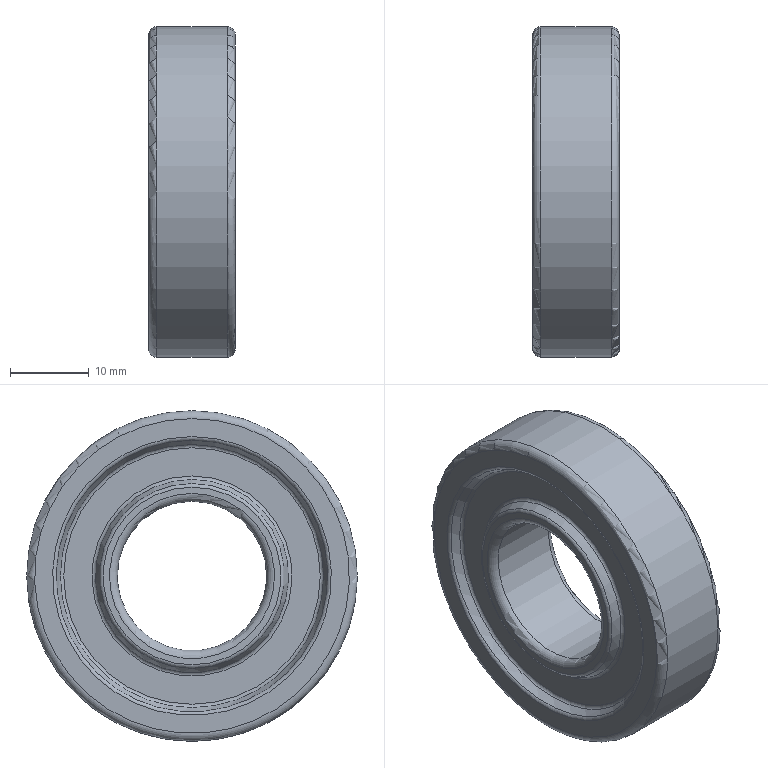Part | STEP file | PL6203ZZA_default | 1 solid | 24 faces | box 11 x 42 x 42 mm | volume 10581 mm3 | torus 12 | plane 6 | cone 4 | cylinder 2 | commonest cylinder face diameters 19 x1 42 x1
STEP:
#1=CARTESIAN_POINT('',(0.,0.,0.));
#2=DIRECTION('',(0.,0.,1.));
#3=DIRECTION('',(1.,0.,0.));
#4=AXIS2_PLACEMENT_3D('',#1,#2,#3);
#5=CARTESIAN_POINT('',(0.,-9.5,20.));
#6=VERTEX_POINT('',#5);
#7=CARTESIAN_POINT('',(0.,-9.5,0.));
#8=DIRECTION('',(-1.,0.,0.));
#9=DIRECTION('',(0.,0.,1.));
#10=AXIS2_PLACEMENT_3D('',#7,#8,#9);
#11=CIRCLE('',#10,20.);
#12=CARTESIAN_POINT('',(1.,-9.5,0.));
#13=DIRECTION('',(-1.,0.,0.));
#14=DIRECTION('',(0.,0.,1.));
#15=AXIS2_PLACEMENT_3D('',#12,#13,#14);
#16=TOROIDAL_SURFACE('',#15,20.,1.);
#17=CARTESIAN_POINT('',(0.,7.854));
#18=DIRECTION('',(1.,0.));
#19=VECTOR('',#18,1.);
#20=LINE('',#17,#19);
#21=(GEOMETRIC_REPRESENTATION_CONTEXT(2)PARAMETRIC_REPRESENTATION_CONTEXT()REPRESENTATION_CONTEXT('',''));
#22=DEFINITIONAL_REPRESENTATION('',(#20),#21);
#23=PCURVE('',#16,#22);
#24=CARTESIAN_POINT('',(0.,8.209,0.));
#25=DIRECTION('',(1.,0.,0.));
#26=DIRECTION('',(0.,0.,-1.));
#27=AXIS2_PLACEMENT_3D('',#24,#25,#26);
#28=PLANE('',#27);
#29=CARTESIAN_POINT('',(-20.,-17.709));
#30=CARTESIAN_POINT('',(-20.,16.932));
#31=CARTESIAN_POINT('',(10.,-0.3885));
#32=CARTESIAN_POINT('',(40.,-17.709));
#33=CARTESIAN_POINT('',(10.,-35.03));
#34=CARTESIAN_POINT('',(-20.,-52.35));
#35=CARTESIAN_POINT('',(-20.,-17.709));
#36=(BOUNDED_CURVE()B_SPLINE_CURVE(2,(#29,#30,#31,#32,#33,#34,#35),.UNSPECIFIED.,.T.,.F.)B_SPLINE_CURVE_WITH_KNOTS((1,2,2,2,2,1),(-2.094,0.,2.094,4.189,6.283,8.378),.UNSPECIFIED.)CURVE()GEOMETRIC_REPRESENTATION_ITEM()RATIONAL_B_SPLINE_CURVE((1.,0.5,1.,0.5,1.,0.5,1.))REPRESENTATION_ITEM(''));
#37=(GEOMETRIC_REPRESENTATION_CONTEXT(2)PARAMETRIC_REPRESENTATION_CONTEXT()REPRESENTATION_CONTEXT('',''));
#38=DEFINITIONAL_REPRESENTATION('',(#36),#37);
#39=PCURVE('',#28,#38);
#40=SURFACE_CURVE('',#11,(#23,#39),.PCURVE_S1.);
#41=EDGE_CURVE('',#6,#6,#40,.T.);
#42=ORIENTED_EDGE('',*,*,#41,.F.);
#43=CARTESIAN_POINT('',(1.,-9.5,21.));
#44=VERTEX_POINT('',#43);
#45=CARTESIAN_POINT('',(1.,-9.5,21.));
#46=CARTESIAN_POINT('',(0.7327,-9.5,21.));
#47=CARTESIAN_POINT('',(0.4723,-9.5,20.915));
#48=CARTESIAN_POINT('',(0.2481,-9.5,20.752));
#49=CARTESIAN_POINT('',(0.085,-9.5,20.528));
#50=CARTESIAN_POINT('',(0.,-9.5,20.267));
#51=CARTESIAN_POINT('',(0.,-9.5,20.));
#52=(BOUNDED_CURVE()B_SPLINE_CURVE(6,(#45,#46,#47,#48,#49,#50,#51),.UNSPECIFIED.,.F.,.F.)B_SPLINE_CURVE_WITH_KNOTS((7,7),(0.,1.571),.PIECEWISE_BEZIER_KNOTS.)CURVE()GEOMETRIC_REPRESENTATION_ITEM()RATIONAL_B_SPLINE_CURVE((1.031,1.01,0.9979,0.994,0.9979,1.01,1.031))REPRESENTATION_ITEM(''));
#53=CARTESIAN_POINT('',(0.,6.283));
#54=DIRECTION('',(0.,1.));
#55=VECTOR('',#54,1.);
#56=LINE('',#53,#55);
#57=(GEOMETRIC_REPRESENTATION_CONTEXT(2)PARAMETRIC_REPRESENTATION_CONTEXT()REPRESENTATION_CONTEXT('',''));
#58=DEFINITIONAL_REPRESENTATION('',(#56),#57);
#59=PCURVE('',#16,#58);
#60=CARTESIAN_POINT('',(6.283,6.283));
#61=DIRECTION('',(0.,1.));
#62=VECTOR('',#61,1.);
#63=LINE('',#60,#62);
#64=(GEOMETRIC_REPRESENTATION_CONTEXT(2)PARAMETRIC_REPRESENTATION_CONTEXT()REPRESENTATION_CONTEXT('',''));
#65=DEFINITIONAL_REPRESENTATION('',(#63),#64);
#66=PCURVE('',#16,#65);
#67=SEAM_CURVE('',#52,(#59,#66),.PCURVE_S1.);
#68=EDGE_CURVE('',#44,#6,#67,.T.);
#69=ORIENTED_EDGE('',*,*,#68,.F.);
#70=CARTESIAN_POINT('',(1.,-9.5,0.));
#71=DIRECTION('',(-1.,0.,0.));
#72=DIRECTION('',(0.,0.,1.));
#73=AXIS2_PLACEMENT_3D('',#70,#71,#72);
#74=CIRCLE('',#73,21.);
#75=CARTESIAN_POINT('',(0.,6.283));
#76=DIRECTION('',(1.,0.));
#77=VECTOR('',#76,1.);
#78=LINE('',#75,#77);
#79=(GEOMETRIC_REPRESENTATION_CONTEXT(2)PARAMETRIC_REPRESENTATION_CONTEXT()REPRESENTATION_CONTEXT('',''));
#80=DEFINITIONAL_REPRESENTATION('',(#78),#79);
#81=PCURVE('',#16,#80);
#82=CARTESIAN_POINT('',(5.5,-9.5,0.));
#83=DIRECTION('',(-1.,0.,0.));
#84=DIRECTION('',(0.,0.,1.));
#85=AXIS2_PLACEMENT_3D('',#82,#83,#84);
#86=CYLINDRICAL_SURFACE('',#85,21.);
#87=CARTESIAN_POINT('',(0.,4.5));
#88=DIRECTION('',(1.,0.));
#89=VECTOR('',#88,1.);
#90=LINE('',#87,#89);
#91=(GEOMETRIC_REPRESENTATION_CONTEXT(2)PARAMETRIC_REPRESENTATION_CONTEXT()REPRESENTATION_CONTEXT('',''));
#92=DEFINITIONAL_REPRESENTATION('',(#90),#91);
#93=PCURVE('',#86,#92);
#94=SURFACE_CURVE('',#74,(#81,#93),.PCURVE_S1.);
#95=EDGE_CURVE('',#44,#44,#94,.T.);
#96=ORIENTED_EDGE('',*,*,#95,.T.);
#97=ORIENTED_EDGE('',*,*,#68,.T.);
#98=EDGE_LOOP('',(#42,#69,#96,#97));
#99=FACE_BOUND('',#98,.T.);
#100=ADVANCED_FACE('',(#99),#16,.T.);
#101=ORIENTED_EDGE('',*,*,#95,.F.);
#102=CARTESIAN_POINT('',(10.,-9.5,21.));
#103=VERTEX_POINT('',#102);
#104=CARTESIAN_POINT('',(10.,-9.5,21.));
#105=CARTESIAN_POINT('',(1.,-9.5,21.));
#106=B_SPLINE_CURVE_WITH_KNOTS('',1,(#104,#105),.UNSPECIFIED.,.F.,.F.,(2,2),(-4.5,4.5),.PIECEWISE_BEZIER_KNOTS.);
#107=CARTESIAN_POINT('',(0.,0.));
#108=DIRECTION('',(0.,1.));
#109=VECTOR('',#108,1.);
#110=LINE('',#107,#109);
#111=(GEOMETRIC_REPRESENTATION_CONTEXT(2)PARAMETRIC_REPRESENTATION_CONTEXT()REPRESENTATION_CONTEXT('',''));
#112=DEFINITIONAL_REPRESENTATION('',(#110),#111);
#113=PCURVE('',#86,#112);
#114=CARTESIAN_POINT('',(6.283,0.));
#115=DIRECTION('',(0.,1.));
#116=VECTOR('',#115,1.);
#117=LINE('',#114,#116);
#118=(GEOMETRIC_REPRESENTATION_CONTEXT(2)PARAMETRIC_REPRESENTATION_CONTEXT()REPRESENTATION_CONTEXT('',''));
#119=DEFINITIONAL_REPRESENTATION('',(#117),#118);
#120=PCURVE('',#86,#119);
#121=SEAM_CURVE('',#106,(#113,#120),.PCURVE_S1.);
#122=EDGE_CURVE('',#103,#44,#121,.T.);
#123=ORIENTED_EDGE('',*,*,#122,.F.);
#124=CARTESIAN_POINT('',(10.,-9.5,0.));
#125=DIRECTION('',(-1.,0.,0.));
#126=DIRECTION('',(0.,0.,1.));
#127=AXIS2_PLACEMENT_3D('',#124,#125,#126);
#128=CIRCLE('',#127,21.);
#129=CARTESIAN_POINT('',(0.,-4.5));
#130=DIRECTION('',(1.,0.));
#131=VECTOR('',#130,1.);
#132=LINE('',#129,#131);
#133=(GEOMETRIC_REPRESENTATION_CONTEXT(2)PARAMETRIC_REPRESENTATION_CONTEXT()REPRESENTATION_CONTEXT('',''));
#134=DEFINITIONAL_REPRESENTATION('',(#132),#133);
#135=PCURVE('',#86,#134);
#136=CARTESIAN_POINT('',(10.,-9.5,0.));
#137=DIRECTION('',(-1.,0.,0.));
#138=DIRECTION('',(0.,0.,1.));
#139=AXIS2_PLACEMENT_3D('',#136,#137,#138);
#140=TOROIDAL_SURFACE('',#139,20.,1.);
#141=CARTESIAN_POINT('',(0.,6.283));
#142=DIRECTION('',(1.,0.));
#143=VECTOR('',#142,1.);
#144=LINE('',#141,#143);
#145=(GEOMETRIC_REPRESENTATION_CONTEXT(2)PARAMETRIC_REPRESENTATION_CONTEXT()REPRESENTATION_CONTEXT('',''));
#146=DEFINITIONAL_REPRESENTATION('',(#144),#145);
#147=PCURVE('',#140,#146);
#148=SURFACE_CURVE('',#128,(#135,#147),.PCURVE_S1.);
#149=EDGE_CURVE('',#103,#103,#148,.T.);
#150=ORIENTED_EDGE('',*,*,#149,.T.);
#151=ORIENTED_EDGE('',*,*,#122,.T.);
#152=EDGE_LOOP('',(#101,#123,#150,#151));
#153=FACE_BOUND('',#152,.T.);
#154=ADVANCED_FACE('',(#153),#86,.T.);
#155=ORIENTED_EDGE('',*,*,#149,.F.);
#156=CARTESIAN_POINT('',(11.,-9.5,20.));
#157=VERTEX_POINT('',#156);
#158=CARTESIAN_POINT('',(11.,-9.5,20.));
#159=CARTESIAN_POINT('',(11.,-9.5,20.267));
#160=CARTESIAN_POINT('',(10.915,-9.5,20.528));
#161=CARTESIAN_POINT('',(10.752,-9.5,20.752));
#162=CARTESIAN_POINT('',(10.528,-9.5,20.915));
#163=CARTESIAN_POINT('',(10.267,-9.5,21.));
#164=CARTESIAN_POINT('',(10.,-9.5,21.));
#165=(BOUNDED_CURVE()B_SPLINE_CURVE(6,(#158,#159,#160,#161,#162,#163,#164),.UNSPECIFIED.,.F.,.F.)B_SPLINE_CURVE_WITH_KNOTS((7,7),(-1.571,0.),.PIECEWISE_BEZIER_KNOTS.)CURVE()GEOMETRIC_REPRESENTATION_ITEM()RATIONAL_B_SPLINE_CURVE((1.031,1.01,0.9979,0.994,0.9979,1.01,1.031))REPRESENTATION_ITEM(''));
#166=CARTESIAN_POINT('',(0.,6.283));
#167=DIRECTION('',(0.,1.));
#168=VECTOR('',#167,1.);
#169=LINE('',#166,#168);
#170=(GEOMETRIC_REPRESENTATION_CONTEXT(2)PARAMETRIC_REPRESENTATION_CONTEXT()REPRESENTATION_CONTEXT('',''));
#171=DEFINITIONAL_REPRESENTATION('',(#169),#170);
#172=PCURVE('',#140,#171);
#173=CARTESIAN_POINT('',(6.283,6.283));
#174=DIRECTION('',(0.,1.));
#175=VECTOR('',#174,1.);
#176=LINE('',#173,#175);
#177=(GEOMETRIC_REPRESENTATION_CONTEXT(2)PARAMETRIC_REPRESENTATION_CONTEXT()REPRESENTATION_CONTEXT('',''));
#178=DEFINITIONAL_REPRESENTATION('',(#176),#177);
#179=PCURVE('',#140,#178);
#180=SEAM_CURVE('',#165,(#172,#179),.PCURVE_S1.);
#181=EDGE_CURVE('',#157,#103,#180,.T.);
#182=ORIENTED_EDGE('',*,*,#181,.F.);
#183=CARTESIAN_POINT('',(11.,-9.5,0.));
#184=DIRECTION('',(-1.,0.,0.));
#185=DIRECTION('',(0.,0.,1.));
#186=AXIS2_PLACEMENT_3D('',#183,#184,#185);
#187=CIRCLE('',#186,20.);
#188=CARTESIAN_POINT('',(0.,4.712));
#189=DIRECTION('',(1.,0.));
#190=VECTOR('',#189,1.);
#191=LINE('',#188,#190);
#192=(GEOMETRIC_REPRESENTATION_CONTEXT(2)PARAMETRIC_REPRESENTATION_CONTEXT()REPRESENTATION_CONTEXT('',''));
#193=DEFINITIONAL_REPRESENTATION('',(#191),#192);
#194=PCURVE('',#140,#193);
#195=CARTESIAN_POINT('',(11.,10.5,0.));
#196=DIRECTION('',(-1.,0.,0.));
#197=DIRECTION('',(0.,0.,1.));
#198=AXIS2_PLACEMENT_3D('',#195,#196,#197);
#199=PLANE('',#198);
#200=CARTESIAN_POINT('',(0.,-20.));
#201=DIRECTION('',(1.,0.));
#202=AXIS2_PLACEMENT_2D('',#200,#201);
#203=CIRCLE('',#202,20.);
#204=(GEOMETRIC_REPRESENTATION_CONTEXT(2)PARAMETRIC_REPRESENTATION_CONTEXT()REPRESENTATION_CONTEXT('',''));
#205=DEFINITIONAL_REPRESENTATION('',(#203),#204);
#206=PCURVE('',#199,#205);
#207=SURFACE_CURVE('',#187,(#194,#206),.PCURVE_S1.);
#208=EDGE_CURVE('',#157,#157,#207,.T.);
#209=ORIENTED_EDGE('',*,*,#208,.T.);
#210=ORIENTED_EDGE('',*,*,#181,.T.);
#211=EDGE_LOOP('',(#155,#182,#209,#210));
#212=FACE_BOUND('',#211,.T.);
#213=ADVANCED_FACE('',(#212),#140,.T.);
#214=ORIENTED_EDGE('',*,*,#208,.F.);
#215=EDGE_LOOP('',(#214));
#216=FACE_BOUND('',#215,.T.);
#217=CARTESIAN_POINT('',(11.,-9.5,17.709));
#218=VERTEX_POINT('',#217);
#219=CARTESIAN_POINT('',(11.,-9.5,0.));
#220=DIRECTION('',(-1.,0.,0.));
#221=DIRECTION('',(0.,0.,1.));
#222=AXIS2_PLACEMENT_3D('',#219,#220,#221);
#223=CIRCLE('',#222,17.709);
#224=CARTESIAN_POINT('',(0.,-20.));
#225=DIRECTION('',(1.,0.));
#226=AXIS2_PLACEMENT_2D('',#224,#225);
#227=CIRCLE('',#226,17.709);
#228=(GEOMETRIC_REPRESENTATION_CONTEXT(2)PARAMETRIC_REPRESENTATION_CONTEXT()REPRESENTATION_CONTEXT('',''));
#229=DEFINITIONAL_REPRESENTATION('',(#227),#228);
#230=PCURVE('',#199,#229);
#231=CARTESIAN_POINT('',(10.5,-9.5,0.));
#232=DIRECTION('',(-1.,0.,0.));
#233=DIRECTION('',(0.,0.,1.));
#234=AXIS2_PLACEMENT_3D('',#231,#232,#233);
#235=TOROIDAL_SURFACE('',#234,17.709,0.5);
#236=CARTESIAN_POINT('',(0.,4.712));
#237=DIRECTION('',(1.,0.));
#238=VECTOR('',#237,1.);
#239=LINE('',#236,#238);
#240=(GEOMETRIC_REPRESENTATION_CONTEXT(2)PARAMETRIC_REPRESENTATION_CONTEXT()REPRESENTATION_CONTEXT('',''));
#241=DEFINITIONAL_REPRESENTATION('',(#239),#240);
#242=PCURVE('',#235,#241);
#243=SURFACE_CURVE('',#223,(#230,#242),.PCURVE_S1.);
#244=EDGE_CURVE('',#218,#218,#243,.T.);
#245=ORIENTED_EDGE('',*,*,#244,.T.);
#246=EDGE_LOOP('',(#245));
#247=FACE_BOUND('',#246,.T.);
#248=ADVANCED_FACE('',(#216,#247),#199,.F.);
#249=ORIENTED_EDGE('',*,*,#244,.F.);
#250=CARTESIAN_POINT('',(10.724,-9.5,17.262));
#251=VERTEX_POINT('',#250);
#252=CARTESIAN_POINT('',(10.724,-9.5,17.262));
#253=CARTESIAN_POINT('',(10.807,-9.5,17.303));
#254=CARTESIAN_POINT('',(10.88,-9.5,17.363));
#255=CARTESIAN_POINT('',(10.939,-9.5,17.438));
#256=CARTESIAN_POINT('',(10.979,-9.5,17.524));
#257=CARTESIAN_POINT('',(11.,-9.5,17.616));
#258=CARTESIAN_POINT('',(11.,-9.5,17.709));
#259=(BOUNDED_CURVE()B_SPLINE_CURVE(6,(#252,#253,#254,#255,#256,#257,#258),.UNSPECIFIED.,.F.,.F.)B_SPLINE_CURVE_WITH_KNOTS((7,7),(3.605,4.712),.PIECEWISE_BEZIER_KNOTS.)CURVE()GEOMETRIC_REPRESENTATION_ITEM()RATIONAL_B_SPLINE_CURVE((1.015,1.005,0.999,0.997,0.999,1.005,1.015))REPRESENTATION_ITEM(''));
#260=CARTESIAN_POINT('',(0.,0.));
#261=DIRECTION('',(0.,1.));
#262=VECTOR('',#261,1.);
#263=LINE('',#260,#262);
#264=(GEOMETRIC_REPRESENTATION_CONTEXT(2)PARAMETRIC_REPRESENTATION_CONTEXT()REPRESENTATION_CONTEXT('',''));
#265=DEFINITIONAL_REPRESENTATION('',(#263),#264);
#266=PCURVE('',#235,#265);
#267=CARTESIAN_POINT('',(6.283,0.));
#268=DIRECTION('',(0.,1.));
#269=VECTOR('',#268,1.);
#270=LINE('',#267,#269);
#271=(GEOMETRIC_REPRESENTATION_CONTEXT(2)PARAMETRIC_REPRESENTATION_CONTEXT()REPRESENTATION_CONTEXT('',''));
#272=DEFINITIONAL_REPRESENTATION('',(#270),#271);
#273=PCURVE('',#235,#272);
#274=SEAM_CURVE('',#259,(#266,#273),.PCURVE_S1.);
#275=EDGE_CURVE('',#251,#218,#274,.T.);
#276=ORIENTED_EDGE('',*,*,#275,.F.);
#277=CARTESIAN_POINT('',(10.724,-9.5,0.));
#278=DIRECTION('',(-1.,0.,0.));
#279=DIRECTION('',(0.,0.,1.));
#280=AXIS2_PLACEMENT_3D('',#277,#278,#279);
#281=CIRCLE('',#280,17.262);
#282=CARTESIAN_POINT('',(0.,3.605));
#283=DIRECTION('',(1.,0.));
#284=VECTOR('',#283,1.);
#285=LINE('',#282,#284);
#286=(GEOMETRIC_REPRESENTATION_CONTEXT(2)PARAMETRIC_REPRESENTATION_CONTEXT()REPRESENTATION_CONTEXT('',''));
#287=DEFINITIONAL_REPRESENTATION('',(#285),#286);
#288=PCURVE('',#235,#287);
#289=CARTESIAN_POINT('',(9.676,-9.5,0.));
#290=DIRECTION('',(1.,0.,0.));
#291=DIRECTION('',(0.,0.,-1.));
#292=AXIS2_PLACEMENT_3D('',#289,#290,#291);
#293=CONICAL_SURFACE('',#292,16.738,0.4636);
#294=CARTESIAN_POINT('',(9.425,1.047));
#295=DIRECTION('',(-1.,0.));
#296=VECTOR('',#295,1.);
#297=LINE('',#294,#296);
#298=(GEOMETRIC_REPRESENTATION_CONTEXT(2)PARAMETRIC_REPRESENTATION_CONTEXT()REPRESENTATION_CONTEXT('',''));
#299=DEFINITIONAL_REPRESENTATION('',(#297),#298);
#300=PCURVE('',#293,#299);
#301=SURFACE_CURVE('',#281,(#288,#300),.PCURVE_S1.);
#302=EDGE_CURVE('',#251,#251,#301,.T.);
#303=ORIENTED_EDGE('',*,*,#302,.T.);
#304=ORIENTED_EDGE('',*,*,#275,.T.);
#305=EDGE_LOOP('',(#249,#276,#303,#304));
#306=FACE_BOUND('',#305,.T.);
#307=ADVANCED_FACE('',(#306),#235,.T.);
#308=ORIENTED_EDGE('',*,*,#302,.T.);
#309=CARTESIAN_POINT('',(9.676,-9.5,16.738));
#310=VERTEX_POINT('',#309);
#311=CARTESIAN_POINT('',(9.676,-9.5,16.738));
#312=CARTESIAN_POINT('',(10.724,-9.5,17.262));
#313=B_SPLINE_CURVE_WITH_KNOTS('',1,(#311,#312),.UNSPECIFIED.,.F.,.F.,(2,2),(0.,1.171),.PIECEWISE_BEZIER_KNOTS.);
#314=CARTESIAN_POINT('',(3.142,0.));
#315=DIRECTION('',(0.,1.));
#316=VECTOR('',#315,1.);
#317=LINE('',#314,#316);
#318=(GEOMETRIC_REPRESENTATION_CONTEXT(2)PARAMETRIC_REPRESENTATION_CONTEXT()REPRESENTATION_CONTEXT('',''));
#319=DEFINITIONAL_REPRESENTATION('',(#317),#318);
#320=PCURVE('',#293,#319);
#321=CARTESIAN_POINT('',(9.425,0.));
#322=DIRECTION('',(0.,1.));
#323=VECTOR('',#322,1.);
#324=LINE('',#321,#323);
#325=(GEOMETRIC_REPRESENTATION_CONTEXT(2)PARAMETRIC_REPRESENTATION_CONTEXT()REPRESENTATION_CONTEXT('',''));
#326=DEFINITIONAL_REPRESENTATION('',(#324),#325);
#327=PCURVE('',#293,#326);
#328=SEAM_CURVE('',#313,(#320,#327),.PCURVE_S1.);
#329=EDGE_CURVE('',#310,#251,#328,.T.);
#330=ORIENTED_EDGE('',*,*,#329,.F.);
#331=CARTESIAN_POINT('',(9.676,-9.5,0.));
#332=DIRECTION('',(-1.,0.,0.));
#333=DIRECTION('',(0.,0.,1.));
#334=AXIS2_PLACEMENT_3D('',#331,#332,#333);
#335=CIRCLE('',#334,16.738);
#336=CARTESIAN_POINT('',(9.425,0.));
#337=DIRECTION('',(-1.,0.));
#338=VECTOR('',#337,1.);
#339=LINE('',#336,#338);
#340=(GEOMETRIC_REPRESENTATION_CONTEXT(2)PARAMETRIC_REPRESENTATION_CONTEXT()REPRESENTATION_CONTEXT('',''));
#341=DEFINITIONAL_REPRESENTATION('',(#339),#340);
#342=PCURVE('',#293,#341);
#343=CARTESIAN_POINT('',(9.9,-9.5,0.));
#344=DIRECTION('',(-1.,0.,0.));
#345=DIRECTION('',(0.,0.,1.));
#346=AXIS2_PLACEMENT_3D('',#343,#344,#345);
#347=TOROIDAL_SURFACE('',#346,16.291,0.5);
#348=CARTESIAN_POINT('',(0.,6.747));
#349=DIRECTION('',(1.,0.));
#350=VECTOR('',#349,1.);
#351=LINE('',#348,#350);
#352=(GEOMETRIC_REPRESENTATION_CONTEXT(2)PARAMETRIC_REPRESENTATION_CONTEXT()REPRESENTATION_CONTEXT('',''));
#353=DEFINITIONAL_REPRESENTATION('',(#351),#352);
#354=PCURVE('',#347,#353);
#355=SURFACE_CURVE('',#335,(#342,#354),.PCURVE_S1.);
#356=EDGE_CURVE('',#310,#310,#355,.T.);
#357=ORIENTED_EDGE('',*,*,#356,.F.);
#358=ORIENTED_EDGE('',*,*,#329,.T.);
#359=EDGE_LOOP('',(#308,#330,#357,#358));
#360=FACE_BOUND('',#359,.F.);
#361=ADVANCED_FACE('',(#360),#293,.F.);
#362=ORIENTED_EDGE('',*,*,#356,.T.);
#363=CARTESIAN_POINT('',(9.4,-9.5,16.291));
#364=VERTEX_POINT('',#363);
#365=CARTESIAN_POINT('',(9.676,-9.5,16.738));
#366=CARTESIAN_POINT('',(9.593,-9.5,16.697));
#367=CARTESIAN_POINT('',(9.52,-9.5,16.637));
#368=CARTESIAN_POINT('',(9.461,-9.5,16.562));
#369=CARTESIAN_POINT('',(9.421,-9.5,16.476));
#370=CARTESIAN_POINT('',(9.4,-9.5,16.384));
#371=CARTESIAN_POINT('',(9.4,-9.5,16.291));
#372=(BOUNDED_CURVE()B_SPLINE_CURVE(6,(#365,#366,#367,#368,#369,#370,#371),.UNSPECIFIED.,.F.,.F.)B_SPLINE_CURVE_WITH_KNOTS((7,7),(0.4636,1.571),.PIECEWISE_BEZIER_KNOTS.)CURVE()GEOMETRIC_REPRESENTATION_ITEM()RATIONAL_B_SPLINE_CURVE((1.015,1.005,0.999,0.997,0.999,1.005,1.015))REPRESENTATION_ITEM(''));
#373=CARTESIAN_POINT('',(6.283,6.283));
#374=DIRECTION('',(0.,1.));
#375=VECTOR('',#374,1.);
#376=LINE('',#373,#375);
#377=(GEOMETRIC_REPRESENTATION_CONTEXT(2)PARAMETRIC_REPRESENTATION_CONTEXT()REPRESENTATION_CONTEXT('',''));
#378=DEFINITIONAL_REPRESENTATION('',(#376),#377);
#379=PCURVE('',#347,#378);
#380=CARTESIAN_POINT('',(0.,6.283));
#381=DIRECTION('',(0.,1.));
#382=VECTOR('',#381,1.);
#383=LINE('',#380,#382);
#384=(GEOMETRIC_REPRESENTATION_CONTEXT(2)PARAMETRIC_REPRESENTATION_CONTEXT()REPRESENTATION_CONTEXT('',''));
#385=DEFINITIONAL_REPRESENTATION('',(#383),#384);
#386=PCURVE('',#347,#385);
#387=SEAM_CURVE('',#372,(#379,#386),.PCURVE_S1.);
#388=EDGE_CURVE('',#310,#364,#387,.T.);
#389=ORIENTED_EDGE('',*,*,#388,.T.);
#390=CARTESIAN_POINT('',(9.4,-9.5,0.));
#391=DIRECTION('',(-1.,0.,0.));
#392=DIRECTION('',(0.,0.,1.));
#393=AXIS2_PLACEMENT_3D('',#390,#391,#392);
#394=CIRCLE('',#393,16.291);
#395=CARTESIAN_POINT('',(0.,7.854));
#396=DIRECTION('',(1.,0.));
#397=VECTOR('',#396,1.);
#398=LINE('',#395,#397);
#399=(GEOMETRIC_REPRESENTATION_CONTEXT(2)PARAMETRIC_REPRESENTATION_CONTEXT()REPRESENTATION_CONTEXT('',''));
#400=DEFINITIONAL_REPRESENTATION('',(#398),#399);
#401=PCURVE('',#347,#400);
#402=CARTESIAN_POINT('',(9.4,6.791,0.));
#403=DIRECTION('',(-1.,0.,0.));
#404=DIRECTION('',(0.,0.,1.));
#405=AXIS2_PLACEMENT_3D('',#402,#403,#404);
#406=PLANE('',#405);
#407=CARTESIAN_POINT('',(0.,-16.291));
#408=DIRECTION('',(1.,0.));
#409=AXIS2_PLACEMENT_2D('',#407,#408);
#410=CIRCLE('',#409,16.291);
#411=(GEOMETRIC_REPRESENTATION_CONTEXT(2)PARAMETRIC_REPRESENTATION_CONTEXT()REPRESENTATION_CONTEXT('',''));
#412=DEFINITIONAL_REPRESENTATION('',(#410),#411);
#413=PCURVE('',#406,#412);
#414=SURFACE_CURVE('',#394,(#401,#413),.PCURVE_S1.);
#415=EDGE_CURVE('',#364,#364,#414,.T.);
#416=ORIENTED_EDGE('',*,*,#415,.F.);
#417=ORIENTED_EDGE('',*,*,#388,.F.);
#418=EDGE_LOOP('',(#362,#389,#416,#417));
#419=FACE_BOUND('',#418,.F.);
#420=ADVANCED_FACE('',(#419),#347,.F.);
#421=ORIENTED_EDGE('',*,*,#415,.F.);
#422=EDGE_LOOP('',(#421));
#423=FACE_BOUND('',#422,.T.);
#424=CARTESIAN_POINT('',(9.4,-9.5,12.709));
#425=VERTEX_POINT('',#424);
#426=CARTESIAN_POINT('',(9.4,-9.5,0.));
#427=DIRECTION('',(-1.,0.,0.));
#428=DIRECTION('',(0.,0.,1.));
#429=AXIS2_PLACEMENT_3D('',#426,#427,#428);
#430=CIRCLE('',#429,12.709);
#431=CARTESIAN_POINT('',(0.,-16.291));
#432=DIRECTION('',(1.,0.));
#433=AXIS2_PLACEMENT_2D('',#431,#432);
#434=CIRCLE('',#433,12.709);
#435=(GEOMETRIC_REPRESENTATION_CONTEXT(2)PARAMETRIC_REPRESENTATION_CONTEXT()REPRESENTATION_CONTEXT('',''));
#436=DEFINITIONAL_REPRESENTATION('',(#434),#435);
#437=PCURVE('',#406,#436);
#438=CARTESIAN_POINT('',(9.9,-9.5,0.));
#439=DIRECTION('',(-1.,0.,0.));
#440=DIRECTION('',(0.,0.,1.));
#441=AXIS2_PLACEMENT_3D('',#438,#439,#440);
#442=TOROIDAL_SURFACE('',#441,12.709,0.5);
#443=CARTESIAN_POINT('',(0.,7.854));
#444=DIRECTION('',(1.,0.));
#445=VECTOR('',#444,1.);
#446=LINE('',#443,#445);
#447=(GEOMETRIC_REPRESENTATION_CONTEXT(2)PARAMETRIC_REPRESENTATION_CONTEXT()REPRESENTATION_CONTEXT('',''));
#448=DEFINITIONAL_REPRESENTATION('',(#446),#447);
#449=PCURVE('',#442,#448);
#450=SURFACE_CURVE('',#430,(#437,#449),.PCURVE_S1.);
#451=EDGE_CURVE('',#425,#425,#450,.T.);
#452=ORIENTED_EDGE('',*,*,#451,.T.);
#453=EDGE_LOOP('',(#452));
#454=FACE_BOUND('',#453,.T.);
#455=ADVANCED_FACE('',(#423,#454),#406,.F.);
#456=ORIENTED_EDGE('',*,*,#451,.T.);
#457=CARTESIAN_POINT('',(9.676,-9.5,12.262));
#458=VERTEX_POINT('',#457);
#459=CARTESIAN_POINT('',(9.4,-9.5,12.709));
#460=CARTESIAN_POINT('',(9.4,-9.5,12.616));
#461=CARTESIAN_POINT('',(9.421,-9.5,12.524));
#462=CARTESIAN_POINT('',(9.461,-9.5,12.438));
#463=CARTESIAN_POINT('',(9.52,-9.5,12.363));
#464=CARTESIAN_POINT('',(9.593,-9.5,12.303));
#465=CARTESIAN_POINT('',(9.676,-9.5,12.262));
#466=(BOUNDED_CURVE()B_SPLINE_CURVE(6,(#459,#460,#461,#462,#463,#464,#465),.UNSPECIFIED.,.F.,.F.)B_SPLINE_CURVE_WITH_KNOTS((7,7),(1.571,2.678),.PIECEWISE_BEZIER_KNOTS.)CURVE()GEOMETRIC_REPRESENTATION_ITEM()RATIONAL_B_SPLINE_CURVE((1.015,1.005,0.999,0.997,0.999,1.005,1.015))REPRESENTATION_ITEM(''));
#467=CARTESIAN_POINT('',(6.283,6.283));
#468=DIRECTION('',(0.,1.));
#469=VECTOR('',#468,1.);
#470=LINE('',#467,#469);
#471=(GEOMETRIC_REPRESENTATION_CONTEXT(2)PARAMETRIC_REPRESENTATION_CONTEXT()REPRESENTATION_CONTEXT('',''));
#472=DEFINITIONAL_REPRESENTATION('',(#470),#471);
#473=PCURVE('',#442,#472);
#474=CARTESIAN_POINT('',(0.,6.283));
#475=DIRECTION('',(0.,1.));
#476=VECTOR('',#475,1.);
#477=LINE('',#474,#476);
#478=(GEOMETRIC_REPRESENTATION_CONTEXT(2)PARAMETRIC_REPRESENTATION_CONTEXT()REPRESENTATION_CONTEXT('',''));
#479=DEFINITIONAL_REPRESENTATION('',(#477),#478);
#480=PCURVE('',#442,#479);
#481=SEAM_CURVE('',#466,(#473,#480),.PCURVE_S1.);
#482=EDGE_CURVE('',#425,#458,#481,.T.);
#483=ORIENTED_EDGE('',*,*,#482,.T.);
#484=CARTESIAN_POINT('',(9.676,-9.5,0.));
#485=DIRECTION('',(-1.,0.,0.));
#486=DIRECTION('',(0.,0.,1.));
#487=AXIS2_PLACEMENT_3D('',#484,#485,#486);
#488=CIRCLE('',#487,12.262);
#489=CARTESIAN_POINT('',(0.,8.961));
#490=DIRECTION('',(1.,0.));
#491=VECTOR('',#490,1.);
#492=LINE('',#489,#491);
#493=(GEOMETRIC_REPRESENTATION_CONTEXT(2)PARAMETRIC_REPRESENTATION_CONTEXT()REPRESENTATION_CONTEXT('',''));
#494=DEFINITIONAL_REPRESENTATION('',(#492),#493);
#495=PCURVE('',#442,#494);
#496=CARTESIAN_POINT('',(10.724,-9.5,0.));
#497=DIRECTION('',(-1.,0.,0.));
#498=DIRECTION('',(0.,0.,1.));
#499=AXIS2_PLACEMENT_3D('',#496,#497,#498);
#500=CONICAL_SURFACE('',#499,11.738,0.4636);
#501=CARTESIAN_POINT('',(0.,1.047));
#502=DIRECTION('',(1.,0.));
#503=VECTOR('',#502,1.);
#504=LINE('',#501,#503);
#505=(GEOMETRIC_REPRESENTATION_CONTEXT(2)PARAMETRIC_REPRESENTATION_CONTEXT()REPRESENTATION_CONTEXT('',''));
#506=DEFINITIONAL_REPRESENTATION('',(#504),#505);
#507=PCURVE('',#500,#506);
#508=SURFACE_CURVE('',#488,(#495,#507),.PCURVE_S1.);
#509=EDGE_CURVE('',#458,#458,#508,.T.);
#510=ORIENTED_EDGE('',*,*,#509,.F.);
#511=ORIENTED_EDGE('',*,*,#482,.F.);
#512=EDGE_LOOP('',(#456,#483,#510,#511));
#513=FACE_BOUND('',#512,.F.);
#514=ADVANCED_FACE('',(#513),#442,.F.);
#515=ORIENTED_EDGE('',*,*,#509,.F.);
#516=CARTESIAN_POINT('',(10.724,-9.5,11.738));
#517=VERTEX_POINT('',#516);
#518=CARTESIAN_POINT('',(10.724,-9.5,11.738));
#519=CARTESIAN_POINT('',(9.676,-9.5,12.262));
#520=B_SPLINE_CURVE_WITH_KNOTS('',1,(#518,#519),.UNSPECIFIED.,.F.,.F.,(2,2),(0.,1.171),.PIECEWISE_BEZIER_KNOTS.);
#521=CARTESIAN_POINT('',(0.,0.));
#522=DIRECTION('',(0.,1.));
#523=VECTOR('',#522,1.);
#524=LINE('',#521,#523);
#525=(GEOMETRIC_REPRESENTATION_CONTEXT(2)PARAMETRIC_REPRESENTATION_CONTEXT()REPRESENTATION_CONTEXT('',''));
#526=DEFINITIONAL_REPRESENTATION('',(#524),#525);
#527=PCURVE('',#500,#526);
#528=CARTESIAN_POINT('',(6.283,0.));
#529=DIRECTION('',(0.,1.));
#530=VECTOR('',#529,1.);
#531=LINE('',#528,#530);
#532=(GEOMETRIC_REPRESENTATION_CONTEXT(2)PARAMETRIC_REPRESENTATION_CONTEXT()REPRESENTATION_CONTEXT('',''));
#533=DEFINITIONAL_REPRESENTATION('',(#531),#532);
#534=PCURVE('',#500,#533);
#535=SEAM_CURVE('',#520,(#527,#534),.PCURVE_S1.);
#536=EDGE_CURVE('',#517,#458,#535,.T.);
#537=ORIENTED_EDGE('',*,*,#536,.F.);
#538=CARTESIAN_POINT('',(10.724,-9.5,0.));
#539=DIRECTION('',(-1.,0.,0.));
#540=DIRECTION('',(0.,0.,1.));
#541=AXIS2_PLACEMENT_3D('',#538,#539,#540);
#542=CIRCLE('',#541,11.738);
#543=CARTESIAN_POINT('',(0.,0.));
#544=DIRECTION('',(1.,0.));
#545=VECTOR('',#544,1.);
#546=LINE('',#543,#545);
#547=(GEOMETRIC_REPRESENTATION_CONTEXT(2)PARAMETRIC_REPRESENTATION_CONTEXT()REPRESENTATION_CONTEXT('',''));
#548=DEFINITIONAL_REPRESENTATION('',(#546),#547);
#549=PCURVE('',#500,#548);
#550=CARTESIAN_POINT('',(10.5,-9.5,0.));
#551=DIRECTION('',(-1.,0.,0.));
#552=DIRECTION('',(0.,0.,1.));
#553=AXIS2_PLACEMENT_3D('',#550,#551,#552);
#554=TOROIDAL_SURFACE('',#553,11.291,0.5);
#555=CARTESIAN_POINT('',(0.,5.82));
#556=DIRECTION('',(1.,0.));
#557=VECTOR('',#556,1.);
#558=LINE('',#555,#557);
#559=(GEOMETRIC_REPRESENTATION_CONTEXT(2)PARAMETRIC_REPRESENTATION_CONTEXT()REPRESENTATION_CONTEXT('',''));
#560=DEFINITIONAL_REPRESENTATION('',(#558),#559);
#561=PCURVE('',#554,#560);
#562=SURFACE_CURVE('',#542,(#549,#561),.PCURVE_S1.);
#563=EDGE_CURVE('',#517,#517,#562,.T.);
#564=ORIENTED_EDGE('',*,*,#563,.T.);
#565=ORIENTED_EDGE('',*,*,#536,.T.);
#566=EDGE_LOOP('',(#515,#537,#564,#565));
#567=FACE_BOUND('',#566,.T.);
#568=ADVANCED_FACE('',(#567),#500,.T.);
#569=ORIENTED_EDGE('',*,*,#563,.F.);
#570=CARTESIAN_POINT('',(11.,-9.5,11.291));
#571=VERTEX_POINT('',#570);
#572=CARTESIAN_POINT('',(11.,-9.5,11.291));
#573=CARTESIAN_POINT('',(11.,-9.5,11.384));
#574=CARTESIAN_POINT('',(10.979,-9.5,11.476));
#575=CARTESIAN_POINT('',(10.939,-9.5,11.562));
#576=CARTESIAN_POINT('',(10.88,-9.5,11.637));
#577=CARTESIAN_POINT('',(10.807,-9.5,11.697));
#578=CARTESIAN_POINT('',(10.724,-9.5,11.738));
#579=(BOUNDED_CURVE()B_SPLINE_CURVE(6,(#572,#573,#574,#575,#576,#577,#578),.UNSPECIFIED.,.F.,.F.)B_SPLINE_CURVE_WITH_KNOTS((7,7),(4.712,5.82),.PIECEWISE_BEZIER_KNOTS.)CURVE()GEOMETRIC_REPRESENTATION_ITEM()RATIONAL_B_SPLINE_CURVE((1.015,1.005,0.999,0.997,0.999,1.005,1.015))REPRESENTATION_ITEM(''));
#580=CARTESIAN_POINT('',(0.,0.));
#581=DIRECTION('',(0.,1.));
#582=VECTOR('',#581,1.);
#583=LINE('',#580,#582);
#584=(GEOMETRIC_REPRESENTATION_CONTEXT(2)PARAMETRIC_REPRESENTATION_CONTEXT()REPRESENTATION_CONTEXT('',''));
#585=DEFINITIONAL_REPRESENTATION('',(#583),#584);
#586=PCURVE('',#554,#585);
#587=CARTESIAN_POINT('',(6.283,0.));
#588=DIRECTION('',(0.,1.));
#589=VECTOR('',#588,1.);
#590=LINE('',#587,#589);
#591=(GEOMETRIC_REPRESENTATION_CONTEXT(2)PARAMETRIC_REPRESENTATION_CONTEXT()REPRESENTATION_CONTEXT('',''));
#592=DEFINITIONAL_REPRESENTATION('',(#590),#591);
#593=PCURVE('',#554,#592);
#594=SEAM_CURVE('',#579,(#586,#593),.PCURVE_S1.);
#595=EDGE_CURVE('',#571,#517,#594,.T.);
#596=ORIENTED_EDGE('',*,*,#595,.F.);
#597=CARTESIAN_POINT('',(11.,-9.5,0.));
#598=DIRECTION('',(-1.,0.,0.));
#599=DIRECTION('',(0.,0.,1.));
#600=AXIS2_PLACEMENT_3D('',#597,#598,#599);
#601=CIRCLE('',#600,11.291);
#602=CARTESIAN_POINT('',(0.,4.712));
#603=DIRECTION('',(1.,0.));
#604=VECTOR('',#603,1.);
#605=LINE('',#602,#604);
#606=(GEOMETRIC_REPRESENTATION_CONTEXT(2)PARAMETRIC_REPRESENTATION_CONTEXT()REPRESENTATION_CONTEXT('',''));
#607=DEFINITIONAL_REPRESENTATION('',(#605),#606);
#608=PCURVE('',#554,#607);
#609=CARTESIAN_POINT('',(11.,1.791,0.));
#610=DIRECTION('',(-1.,0.,0.));
#611=DIRECTION('',(0.,0.,1.));
#612=AXIS2_PLACEMENT_3D('',#609,#610,#611);
#613=PLANE('',#612);
#614=CARTESIAN_POINT('',(0.,-11.291));
#615=DIRECTION('',(1.,0.));
#616=AXIS2_PLACEMENT_2D('',#614,#615);
#617=CIRCLE('',#616,11.291);
#618=(GEOMETRIC_REPRESENTATION_CONTEXT(2)PARAMETRIC_REPRESENTATION_CONTEXT()REPRESENTATION_CONTEXT('',''));
#619=DEFINITIONAL_REPRESENTATION('',(#617),#618);
#620=PCURVE('',#613,#619);
#621=SURFACE_CURVE('',#601,(#608,#620),.PCURVE_S1.);
#622=EDGE_CURVE('',#571,#571,#621,.T.);
#623=ORIENTED_EDGE('',*,*,#622,.T.);
#624=ORIENTED_EDGE('',*,*,#595,.T.);
#625=EDGE_LOOP('',(#569,#596,#623,#624));
#626=FACE_BOUND('',#625,.T.);
#627=ADVANCED_FACE('',(#626),#554,.T.);
#628=ORIENTED_EDGE('',*,*,#622,.F.);
#629=EDGE_LOOP('',(#628));
#630=FACE_BOUND('',#629,.T.);
#631=CARTESIAN_POINT('',(11.,-9.5,10.5));
#632=VERTEX_POINT('',#631);
#633=CARTESIAN_POINT('',(11.,-9.5,0.));
#634=DIRECTION('',(-1.,0.,0.));
#635=DIRECTION('',(0.,0.,1.));
#636=AXIS2_PLACEMENT_3D('',#633,#634,#635);
#637=CIRCLE('',#636,10.5);
#638=CARTESIAN_POINT('',(0.,-11.291));
#639=DIRECTION('',(1.,0.));
#640=AXIS2_PLACEMENT_2D('',#638,#639);
#641=CIRCLE('',#640,10.5);
#642=(GEOMETRIC_REPRESENTATION_CONTEXT(2)PARAMETRIC_REPRESENTATION_CONTEXT()REPRESENTATION_CONTEXT('',''));
#643=DEFINITIONAL_REPRESENTATION('',(#641),#642);
#644=PCURVE('',#613,#643);
#645=CARTESIAN_POINT('',(10.,-9.5,0.));
#646=DIRECTION('',(-1.,0.,0.));
#647=DIRECTION('',(0.,0.,1.));
#648=AXIS2_PLACEMENT_3D('',#645,#646,#647);
#649=TOROIDAL_SURFACE('',#648,10.5,1.);
#650=CARTESIAN_POINT('',(0.,4.712));
#651=DIRECTION('',(1.,0.));
#652=VECTOR('',#651,1.);
#653=LINE('',#650,#652);
#654=(GEOMETRIC_REPRESENTATION_CONTEXT(2)PARAMETRIC_REPRESENTATION_CONTEXT()REPRESENTATION_CONTEXT('',''));
#655=DEFINITIONAL_REPRESENTATION('',(#653),#654);
#656=PCURVE('',#649,#655);
#657=SURFACE_CURVE('',#637,(#644,#656),.PCURVE_S1.);
#658=EDGE_CURVE('',#632,#632,#657,.T.);
#659=ORIENTED_EDGE('',*,*,#658,.T.);
#660=EDGE_LOOP('',(#659));
#661=FACE_BOUND('',#660,.T.);
#662=ADVANCED_FACE('',(#630,#661),#613,.F.);
#663=ORIENTED_EDGE('',*,*,#658,.F.);
#664=CARTESIAN_POINT('',(10.,-9.5,9.5));
#665=VERTEX_POINT('',#664);
#666=CARTESIAN_POINT('',(10.,-9.5,9.5));
#667=CARTESIAN_POINT('',(10.267,-9.5,9.5));
#668=CARTESIAN_POINT('',(10.528,-9.5,9.585));
#669=CARTESIAN_POINT('',(10.752,-9.5,9.748));
#670=CARTESIAN_POINT('',(10.915,-9.5,9.972));
#671=CARTESIAN_POINT('',(11.,-9.5,10.233));
#672=CARTESIAN_POINT('',(11.,-9.5,10.5));
#673=(BOUNDED_CURVE()B_SPLINE_CURVE(6,(#666,#667,#668,#669,#670,#671,#672),.UNSPECIFIED.,.F.,.F.)B_SPLINE_CURVE_WITH_KNOTS((7,7),(3.142,4.712),.PIECEWISE_BEZIER_KNOTS.)CURVE()GEOMETRIC_REPRESENTATION_ITEM()RATIONAL_B_SPLINE_CURVE((1.031,1.01,0.9979,0.994,0.9979,1.01,1.031))REPRESENTATION_ITEM(''));
#674=CARTESIAN_POINT('',(0.,0.));
#675=DIRECTION('',(0.,1.));
#676=VECTOR('',#675,1.);
#677=LINE('',#674,#676);
#678=(GEOMETRIC_REPRESENTATION_CONTEXT(2)PARAMETRIC_REPRESENTATION_CONTEXT()REPRESENTATION_CONTEXT('',''));
#679=DEFINITIONAL_REPRESENTATION('',(#677),#678);
#680=PCURVE('',#649,#679);
#681=CARTESIAN_POINT('',(6.283,0.));
#682=DIRECTION('',(0.,1.));
#683=VECTOR('',#682,1.);
#684=LINE('',#681,#683);
#685=(GEOMETRIC_REPRESENTATION_CONTEXT(2)PARAMETRIC_REPRESENTATION_CONTEXT()REPRESENTATION_CONTEXT('',''));
#686=DEFINITIONAL_REPRESENTATION('',(#684),#685);
#687=PCURVE('',#649,#686);
#688=SEAM_CURVE('',#673,(#680,#687),.PCURVE_S1.);
#689=EDGE_CURVE('',#665,#632,#688,.T.);
#690=ORIENTED_EDGE('',*,*,#689,.F.);
#691=CARTESIAN_POINT('',(10.,-9.5,0.));
#692=DIRECTION('',(-1.,0.,0.));
#693=DIRECTION('',(0.,0.,1.));
#694=AXIS2_PLACEMENT_3D('',#691,#692,#693);
#695=CIRCLE('',#694,9.5);
#696=CARTESIAN_POINT('',(0.,3.142));
#697=DIRECTION('',(1.,0.));
#698=VECTOR('',#697,1.);
#699=LINE('',#696,#698);
#700=(GEOMETRIC_REPRESENTATION_CONTEXT(2)PARAMETRIC_REPRESENTATION_CONTEXT()REPRESENTATION_CONTEXT('',''));
#701=DEFINITIONAL_REPRESENTATION('',(#699),#700);
#702=PCURVE('',#649,#701);
#703=CARTESIAN_POINT('',(5.5,-9.5,0.));
#704=DIRECTION('',(-1.,0.,0.));
#705=DIRECTION('',(0.,0.,1.));
#706=AXIS2_PLACEMENT_3D('',#703,#704,#705);
#707=CYLINDRICAL_SURFACE('',#706,9.5);
#708=CARTESIAN_POINT('',(0.,-4.5));
#709=DIRECTION('',(1.,0.));
#710=VECTOR('',#709,1.);
#711=LINE('',#708,#710);
#712=(GEOMETRIC_REPRESENTATION_CONTEXT(2)PARAMETRIC_REPRESENTATION_CONTEXT()REPRESENTATION_CONTEXT('',''));
#713=DEFINITIONAL_REPRESENTATION('',(#711),#712);
#714=PCURVE('',#707,#713);
#715=SURFACE_CURVE('',#695,(#702,#714),.PCURVE_S1.);
#716=EDGE_CURVE('',#665,#665,#715,.T.);
#717=ORIENTED_EDGE('',*,*,#716,.T.);
#718=ORIENTED_EDGE('',*,*,#689,.T.);
#719=EDGE_LOOP('',(#663,#690,#717,#718));
#720=FACE_BOUND('',#719,.T.);
#721=ADVANCED_FACE('',(#720),#649,.T.);
#722=ORIENTED_EDGE('',*,*,#716,.T.);
#723=CARTESIAN_POINT('',(1.,-9.5,9.5));
#724=VERTEX_POINT('',#723);
#725=CARTESIAN_POINT('',(10.,-9.5,9.5));
#726=CARTESIAN_POINT('',(1.,-9.5,9.5));
#727=B_SPLINE_CURVE_WITH_KNOTS('',1,(#725,#726),.UNSPECIFIED.,.F.,.F.,(2,2),(-4.5,4.5),.PIECEWISE_BEZIER_KNOTS.);
#728=CARTESIAN_POINT('',(6.283,0.));
#729=DIRECTION('',(0.,1.));
#730=VECTOR('',#729,1.);
#731=LINE('',#728,#730);
#732=(GEOMETRIC_REPRESENTATION_CONTEXT(2)PARAMETRIC_REPRESENTATION_CONTEXT()REPRESENTATION_CONTEXT('',''));
#733=DEFINITIONAL_REPRESENTATION('',(#731),#732);
#734=PCURVE('',#707,#733);
#735=CARTESIAN_POINT('',(0.,0.));
#736=DIRECTION('',(0.,1.));
#737=VECTOR('',#736,1.);
#738=LINE('',#735,#737);
#739=(GEOMETRIC_REPRESENTATION_CONTEXT(2)PARAMETRIC_REPRESENTATION_CONTEXT()REPRESENTATION_CONTEXT('',''));
#740=DEFINITIONAL_REPRESENTATION('',(#738),#739);
#741=PCURVE('',#707,#740);
#742=SEAM_CURVE('',#727,(#734,#741),.PCURVE_S1.);
#743=EDGE_CURVE('',#665,#724,#742,.T.);
#744=ORIENTED_EDGE('',*,*,#743,.T.);
#745=CARTESIAN_POINT('',(1.,-9.5,0.));
#746=DIRECTION('',(-1.,0.,0.));
#747=DIRECTION('',(0.,0.,1.));
#748=AXIS2_PLACEMENT_3D('',#745,#746,#747);
#749=CIRCLE('',#748,9.5);
#750=CARTESIAN_POINT('',(0.,4.5));
#751=DIRECTION('',(1.,0.));
#752=VECTOR('',#751,1.);
#753=LINE('',#750,#752);
#754=(GEOMETRIC_REPRESENTATION_CONTEXT(2)PARAMETRIC_REPRESENTATION_CONTEXT()REPRESENTATION_CONTEXT('',''));
#755=DEFINITIONAL_REPRESENTATION('',(#753),#754);
#756=PCURVE('',#707,#755);
#757=CARTESIAN_POINT('',(1.,-9.5,0.));
#758=DIRECTION('',(-1.,0.,0.));
#759=DIRECTION('',(0.,0.,1.));
#760=AXIS2_PLACEMENT_3D('',#757,#758,#759);
#761=TOROIDAL_SURFACE('',#760,10.5,1.);
#762=CARTESIAN_POINT('',(0.,9.425));
#763=DIRECTION('',(1.,0.));
#764=VECTOR('',#763,1.);
#765=LINE('',#762,#764);
#766=(GEOMETRIC_REPRESENTATION_CONTEXT(2)PARAMETRIC_REPRESENTATION_CONTEXT()REPRESENTATION_CONTEXT('',''));
#767=DEFINITIONAL_REPRESENTATION('',(#765),#766);
#768=PCURVE('',#761,#767);
#769=SURFACE_CURVE('',#749,(#756,#768),.PCURVE_S1.);
#770=EDGE_CURVE('',#724,#724,#769,.T.);
#771=ORIENTED_EDGE('',*,*,#770,.F.);
#772=ORIENTED_EDGE('',*,*,#743,.F.);
#773=EDGE_LOOP('',(#722,#744,#771,#772));
#774=FACE_BOUND('',#773,.F.);
#775=ADVANCED_FACE('',(#774),#707,.F.);
#776=ORIENTED_EDGE('',*,*,#770,.F.);
#777=CARTESIAN_POINT('',(0.,-9.5,10.5));
#778=VERTEX_POINT('',#777);
#779=CARTESIAN_POINT('',(0.,-9.5,10.5));
#780=CARTESIAN_POINT('',(0.,-9.5,10.233));
#781=CARTESIAN_POINT('',(0.085,-9.5,9.972));
#782=CARTESIAN_POINT('',(0.2481,-9.5,9.748));
#783=CARTESIAN_POINT('',(0.4723,-9.5,9.585));
#784=CARTESIAN_POINT('',(0.7327,-9.5,9.5));
#785=CARTESIAN_POINT('',(1.,-9.5,9.5));
#786=(BOUNDED_CURVE()B_SPLINE_CURVE(6,(#779,#780,#781,#782,#783,#784,#785),.UNSPECIFIED.,.F.,.F.)B_SPLINE_CURVE_WITH_KNOTS((7,7),(1.571,3.142),.PIECEWISE_BEZIER_KNOTS.)CURVE()GEOMETRIC_REPRESENTATION_ITEM()RATIONAL_B_SPLINE_CURVE((1.031,1.01,0.9979,0.994,0.9979,1.01,1.031))REPRESENTATION_ITEM(''));
#787=CARTESIAN_POINT('',(0.,6.283));
#788=DIRECTION('',(0.,1.));
#789=VECTOR('',#788,1.);
#790=LINE('',#787,#789);
#791=(GEOMETRIC_REPRESENTATION_CONTEXT(2)PARAMETRIC_REPRESENTATION_CONTEXT()REPRESENTATION_CONTEXT('',''));
#792=DEFINITIONAL_REPRESENTATION('',(#790),#791);
#793=PCURVE('',#761,#792);
#794=CARTESIAN_POINT('',(6.283,6.283));
#795=DIRECTION('',(0.,1.));
#796=VECTOR('',#795,1.);
#797=LINE('',#794,#796);
#798=(GEOMETRIC_REPRESENTATION_CONTEXT(2)PARAMETRIC_REPRESENTATION_CONTEXT()REPRESENTATION_CONTEXT('',''));
#799=DEFINITIONAL_REPRESENTATION('',(#797),#798);
#800=PCURVE('',#761,#799);
#801=SEAM_CURVE('',#786,(#793,#800),.PCURVE_S1.);
#802=EDGE_CURVE('',#778,#724,#801,.T.);
#803=ORIENTED_EDGE('',*,*,#802,.F.);
#804=CARTESIAN_POINT('',(0.,-9.5,0.));
#805=DIRECTION('',(-1.,0.,0.));
#806=DIRECTION('',(0.,0.,1.));
#807=AXIS2_PLACEMENT_3D('',#804,#805,#806);
#808=CIRCLE('',#807,10.5);
#809=CARTESIAN_POINT('',(0.,7.854));
#810=DIRECTION('',(1.,0.));
#811=VECTOR('',#810,1.);
#812=LINE('',#809,#811);
#813=(GEOMETRIC_REPRESENTATION_CONTEXT(2)PARAMETRIC_REPRESENTATION_CONTEXT()REPRESENTATION_CONTEXT('',''));
#814=DEFINITIONAL_REPRESENTATION('',(#812),#813);
#815=PCURVE('',#761,#814);
#816=CARTESIAN_POINT('',(0.,1.,0.));
#817=DIRECTION('',(1.,0.,0.));
#818=DIRECTION('',(0.,0.,-1.));
#819=AXIS2_PLACEMENT_3D('',#816,#817,#818);
#820=PLANE('',#819);
#821=CARTESIAN_POINT('',(-10.5,-10.5));
#822=CARTESIAN_POINT('',(-10.5,7.687));
#823=CARTESIAN_POINT('',(5.25,-1.407));
#824=CARTESIAN_POINT('',(21.,-10.5));
#825=CARTESIAN_POINT('',(5.25,-19.593));
#826=CARTESIAN_POINT('',(-10.5,-28.687));
#827=CARTESIAN_POINT('',(-10.5,-10.5));
#828=(BOUNDED_CURVE()B_SPLINE_CURVE(2,(#821,#822,#823,#824,#825,#826,#827),.UNSPECIFIED.,.T.,.F.)B_SPLINE_CURVE_WITH_KNOTS((1,2,2,2,2,1),(-2.094,0.,2.094,4.189,6.283,8.378),.UNSPECIFIED.)CURVE()GEOMETRIC_REPRESENTATION_ITEM()RATIONAL_B_SPLINE_CURVE((1.,0.5,1.,0.5,1.,0.5,1.))REPRESENTATION_ITEM(''));
#829=(GEOMETRIC_REPRESENTATION_CONTEXT(2)PARAMETRIC_REPRESENTATION_CONTEXT()REPRESENTATION_CONTEXT('',''));
#830=DEFINITIONAL_REPRESENTATION('',(#828),#829);
#831=PCURVE('',#820,#830);
#832=SURFACE_CURVE('',#808,(#815,#831),.PCURVE_S1.);
#833=EDGE_CURVE('',#778,#778,#832,.T.);
#834=ORIENTED_EDGE('',*,*,#833,.T.);
#835=ORIENTED_EDGE('',*,*,#802,.T.);
#836=EDGE_LOOP('',(#776,#803,#834,#835));
#837=FACE_BOUND('',#836,.T.);
#838=ADVANCED_FACE('',(#837),#761,.T.);
#839=ORIENTED_EDGE('',*,*,#833,.F.);
#840=EDGE_LOOP('',(#839));
#841=FACE_BOUND('',#840,.T.);
#842=CARTESIAN_POINT('',(0.,-9.5,11.291));
#843=VERTEX_POINT('',#842);
#844=CARTESIAN_POINT('',(0.,-9.5,0.));
#845=DIRECTION('',(-1.,0.,0.));
#846=DIRECTION('',(0.,0.,1.));
#847=AXIS2_PLACEMENT_3D('',#844,#845,#846);
#848=CIRCLE('',#847,11.291);
#849=CARTESIAN_POINT('',(-11.291,-10.5));
#850=CARTESIAN_POINT('',(-11.291,9.057));
#851=CARTESIAN_POINT('',(5.645,-0.7217));
#852=CARTESIAN_POINT('',(22.582,-10.5));
#853=CARTESIAN_POINT('',(5.645,-20.278));
#854=CARTESIAN_POINT('',(-11.291,-30.057));
#855=CARTESIAN_POINT('',(-11.291,-10.5));
#856=(BOUNDED_CURVE()B_SPLINE_CURVE(2,(#849,#850,#851,#852,#853,#854,#855),.UNSPECIFIED.,.T.,.F.)B_SPLINE_CURVE_WITH_KNOTS((1,2,2,2,2,1),(-2.094,0.,2.094,4.189,6.283,8.378),.UNSPECIFIED.)CURVE()GEOMETRIC_REPRESENTATION_ITEM()RATIONAL_B_SPLINE_CURVE((1.,0.5,1.,0.5,1.,0.5,1.))REPRESENTATION_ITEM(''));
#857=(GEOMETRIC_REPRESENTATION_CONTEXT(2)PARAMETRIC_REPRESENTATION_CONTEXT()REPRESENTATION_CONTEXT('',''));
#858=DEFINITIONAL_REPRESENTATION('',(#856),#857);
#859=PCURVE('',#820,#858);
#860=CARTESIAN_POINT('',(0.5,-9.5,0.));
#861=DIRECTION('',(-1.,0.,0.));
#862=DIRECTION('',(0.,0.,1.));
#863=AXIS2_PLACEMENT_3D('',#860,#861,#862);
#864=TOROIDAL_SURFACE('',#863,11.291,0.5);
#865=CARTESIAN_POINT('',(0.,7.854));
#866=DIRECTION('',(1.,0.));
#867=VECTOR('',#866,1.);
#868=LINE('',#865,#867);
#869=(GEOMETRIC_REPRESENTATION_CONTEXT(2)PARAMETRIC_REPRESENTATION_CONTEXT()REPRESENTATION_CONTEXT('',''));
#870=DEFINITIONAL_REPRESENTATION('',(#868),#869);
#871=PCURVE('',#864,#870);
#872=SURFACE_CURVE('',#848,(#859,#871),.PCURVE_S1.);
#873=EDGE_CURVE('',#843,#843,#872,.T.);
#874=ORIENTED_EDGE('',*,*,#873,.T.);
#875=EDGE_LOOP('',(#874));
#876=FACE_BOUND('',#875,.T.);
#877=ADVANCED_FACE('',(#841,#876),#820,.F.);
#878=ORIENTED_EDGE('',*,*,#873,.F.);
#879=CARTESIAN_POINT('',(0.2764,-9.5,11.738));
#880=VERTEX_POINT('',#879);
#881=CARTESIAN_POINT('',(0.2764,-9.5,11.738));
#882=CARTESIAN_POINT('',(0.193,-9.5,11.697));
#883=CARTESIAN_POINT('',(0.12,-9.5,11.637));
#884=CARTESIAN_POINT('',(0.06147,-9.5,11.562));
#885=CARTESIAN_POINT('',(0.02077,-9.5,11.476));
#886=CARTESIAN_POINT('',(0.,-9.5,11.384));
#887=CARTESIAN_POINT('',(0.,-9.5,11.291));
#888=(BOUNDED_CURVE()B_SPLINE_CURVE(6,(#881,#882,#883,#884,#885,#886,#887),.UNSPECIFIED.,.F.,.F.)B_SPLINE_CURVE_WITH_KNOTS((7,7),(0.4636,1.571),.PIECEWISE_BEZIER_KNOTS.)CURVE()GEOMETRIC_REPRESENTATION_ITEM()RATIONAL_B_SPLINE_CURVE((1.015,1.005,0.999,0.997,0.999,1.005,1.015))REPRESENTATION_ITEM(''));
#889=CARTESIAN_POINT('',(0.,6.283));
#890=DIRECTION('',(0.,1.));
#891=VECTOR('',#890,1.);
#892=LINE('',#889,#891);
#893=(GEOMETRIC_REPRESENTATION_CONTEXT(2)PARAMETRIC_REPRESENTATION_CONTEXT()REPRESENTATION_CONTEXT('',''));
#894=DEFINITIONAL_REPRESENTATION('',(#892),#893);
#895=PCURVE('',#864,#894);
#896=CARTESIAN_POINT('',(6.283,6.283));
#897=DIRECTION('',(0.,1.));
#898=VECTOR('',#897,1.);
#899=LINE('',#896,#898);
#900=(GEOMETRIC_REPRESENTATION_CONTEXT(2)PARAMETRIC_REPRESENTATION_CONTEXT()REPRESENTATION_CONTEXT('',''));
#901=DEFINITIONAL_REPRESENTATION('',(#899),#900);
#902=PCURVE('',#864,#901);
#903=SEAM_CURVE('',#888,(#895,#902),.PCURVE_S1.);
#904=EDGE_CURVE('',#880,#843,#903,.T.);
#905=ORIENTED_EDGE('',*,*,#904,.F.);
#906=CARTESIAN_POINT('',(0.2764,-9.5,0.));
#907=DIRECTION('',(-1.,0.,0.));
#908=DIRECTION('',(0.,0.,1.));
#909=AXIS2_PLACEMENT_3D('',#906,#907,#908);
#910=CIRCLE('',#909,11.738);
#911=CARTESIAN_POINT('',(0.,6.747));
#912=DIRECTION('',(1.,0.));
#913=VECTOR('',#912,1.);
#914=LINE('',#911,#913);
#915=(GEOMETRIC_REPRESENTATION_CONTEXT(2)PARAMETRIC_REPRESENTATION_CONTEXT()REPRESENTATION_CONTEXT('',''));
#916=DEFINITIONAL_REPRESENTATION('',(#914),#915);
#917=PCURVE('',#864,#916);
#918=CARTESIAN_POINT('',(1.324,-9.5,0.));
#919=DIRECTION('',(1.,0.,0.));
#920=DIRECTION('',(0.,0.,-1.));
#921=AXIS2_PLACEMENT_3D('',#918,#919,#920);
#922=CONICAL_SURFACE('',#921,12.262,0.4636);
#923=CARTESIAN_POINT('',(9.425,-1.047));
#924=DIRECTION('',(-1.,0.));
#925=VECTOR('',#924,1.);
#926=LINE('',#923,#925);
#927=(GEOMETRIC_REPRESENTATION_CONTEXT(2)PARAMETRIC_REPRESENTATION_CONTEXT()REPRESENTATION_CONTEXT('',''));
#928=DEFINITIONAL_REPRESENTATION('',(#926),#927);
#929=PCURVE('',#922,#928);
#930=SURFACE_CURVE('',#910,(#917,#929),.PCURVE_S1.);
#931=EDGE_CURVE('',#880,#880,#930,.T.);
#932=ORIENTED_EDGE('',*,*,#931,.T.);
#933=ORIENTED_EDGE('',*,*,#904,.T.);
#934=EDGE_LOOP('',(#878,#905,#932,#933));
#935=FACE_BOUND('',#934,.T.);
#936=ADVANCED_FACE('',(#935),#864,.T.);
#937=ORIENTED_EDGE('',*,*,#931,.F.);
#938=CARTESIAN_POINT('',(1.324,-9.5,12.262));
#939=VERTEX_POINT('',#938);
#940=CARTESIAN_POINT('',(0.2764,-9.5,11.738));
#941=CARTESIAN_POINT('',(1.324,-9.5,12.262));
#942=B_SPLINE_CURVE_WITH_KNOTS('',1,(#940,#941),.UNSPECIFIED.,.F.,.F.,(2,2),(-1.171,0.),.PIECEWISE_BEZIER_KNOTS.);
#943=CARTESIAN_POINT('',(9.425,0.));
#944=DIRECTION('',(0.,1.));
#945=VECTOR('',#944,1.);
#946=LINE('',#943,#945);
#947=(GEOMETRIC_REPRESENTATION_CONTEXT(2)PARAMETRIC_REPRESENTATION_CONTEXT()REPRESENTATION_CONTEXT('',''));
#948=DEFINITIONAL_REPRESENTATION('',(#946),#947);
#949=PCURVE('',#922,#948);
#950=CARTESIAN_POINT('',(3.142,0.));
#951=DIRECTION('',(0.,1.));
#952=VECTOR('',#951,1.);
#953=LINE('',#950,#952);
#954=(GEOMETRIC_REPRESENTATION_CONTEXT(2)PARAMETRIC_REPRESENTATION_CONTEXT()REPRESENTATION_CONTEXT('',''));
#955=DEFINITIONAL_REPRESENTATION('',(#953),#954);
#956=PCURVE('',#922,#955);
#957=SEAM_CURVE('',#942,(#949,#956),.PCURVE_S1.);
#958=EDGE_CURVE('',#880,#939,#957,.T.);
#959=ORIENTED_EDGE('',*,*,#958,.T.);
#960=CARTESIAN_POINT('',(1.324,-9.5,0.));
#961=DIRECTION('',(-1.,0.,0.));
#962=DIRECTION('',(0.,0.,1.));
#963=AXIS2_PLACEMENT_3D('',#960,#961,#962);
#964=CIRCLE('',#963,12.262);
#965=CARTESIAN_POINT('',(9.425,0.));
#966=DIRECTION('',(-1.,0.));
#967=VECTOR('',#966,1.);
#968=LINE('',#965,#967);
#969=(GEOMETRIC_REPRESENTATION_CONTEXT(2)PARAMETRIC_REPRESENTATION_CONTEXT()REPRESENTATION_CONTEXT('',''));
#970=DEFINITIONAL_REPRESENTATION('',(#968),#969);
#971=PCURVE('',#922,#970);
#972=CARTESIAN_POINT('',(1.1,-9.5,0.));
#973=DIRECTION('',(-1.,0.,0.));
#974=DIRECTION('',(0.,0.,1.));
#975=AXIS2_PLACEMENT_3D('',#972,#973,#974);
#976=TOROIDAL_SURFACE('',#975,12.709,0.5);
#977=CARTESIAN_POINT('',(0.,3.605));
#978=DIRECTION('',(1.,0.));
#979=VECTOR('',#978,1.);
#980=LINE('',#977,#979);
#981=(GEOMETRIC_REPRESENTATION_CONTEXT(2)PARAMETRIC_REPRESENTATION_CONTEXT()REPRESENTATION_CONTEXT('',''));
#982=DEFINITIONAL_REPRESENTATION('',(#980),#981);
#983=PCURVE('',#976,#982);
#984=SURFACE_CURVE('',#964,(#971,#983),.PCURVE_S1.);
#985=EDGE_CURVE('',#939,#939,#984,.T.);
#986=ORIENTED_EDGE('',*,*,#985,.T.);
#987=ORIENTED_EDGE('',*,*,#958,.F.);
#988=EDGE_LOOP('',(#937,#959,#986,#987));
#989=FACE_BOUND('',#988,.T.);
#990=ADVANCED_FACE('',(#989),#922,.T.);
#991=ORIENTED_EDGE('',*,*,#985,.T.);
#992=CARTESIAN_POINT('',(1.6,-9.5,12.709));
#993=VERTEX_POINT('',#992);
#994=CARTESIAN_POINT('',(1.324,-9.5,12.262));
#995=CARTESIAN_POINT('',(1.407,-9.5,12.303));
#996=CARTESIAN_POINT('',(1.48,-9.5,12.363));
#997=CARTESIAN_POINT('',(1.539,-9.5,12.438));
#998=CARTESIAN_POINT('',(1.579,-9.5,12.524));
#999=CARTESIAN_POINT('',(1.6,-9.5,12.616));
#1000=CARTESIAN_POINT('',(1.6,-9.5,12.709));
#1001=(BOUNDED_CURVE()B_SPLINE_CURVE(6,(#994,#995,#996,#997,#998,#999,#1000),.UNSPECIFIED.,.F.,.F.)B_SPLINE_CURVE_WITH_KNOTS((7,7),(3.605,4.712),.PIECEWISE_BEZIER_KNOTS.)CURVE()GEOMETRIC_REPRESENTATION_ITEM()RATIONAL_B_SPLINE_CURVE((1.015,1.005,0.999,0.997,0.999,1.005,1.015))REPRESENTATION_ITEM(''));
#1002=CARTESIAN_POINT('',(6.283,0.));
#1003=DIRECTION('',(0.,1.));
#1004=VECTOR('',#1003,1.);
#1005=LINE('',#1002,#1004);
#1006=(GEOMETRIC_REPRESENTATION_CONTEXT(2)PARAMETRIC_REPRESENTATION_CONTEXT()REPRESENTATION_CONTEXT('',''));
#1007=DEFINITIONAL_REPRESENTATION('',(#1005),#1006);
#1008=PCURVE('',#976,#1007);
#1009=CARTESIAN_POINT('',(0.,0.));
#1010=DIRECTION('',(0.,1.));
#1011=VECTOR('',#1010,1.);
#1012=LINE('',#1009,#1011);
#1013=(GEOMETRIC_REPRESENTATION_CONTEXT(2)PARAMETRIC_REPRESENTATION_CONTEXT()REPRESENTATION_CONTEXT('',''));
#1014=DEFINITIONAL_REPRESENTATION('',(#1012),#1013);
#1015=PCURVE('',#976,#1014);
#1016=SEAM_CURVE('',#1001,(#1008,#1015),.PCURVE_S1.);
#1017=EDGE_CURVE('',#939,#993,#1016,.T.);
#1018=ORIENTED_EDGE('',*,*,#1017,.T.);
#1019=CARTESIAN_POINT('',(1.6,-9.5,0.));
#1020=DIRECTION('',(-1.,0.,0.));
#1021=DIRECTION('',(0.,0.,1.));
#1022=AXIS2_PLACEMENT_3D('',#1019,#1020,#1021);
#1023=CIRCLE('',#1022,12.709);
#1024=CARTESIAN_POINT('',(0.,4.712));
#1025=DIRECTION('',(1.,0.));
#1026=VECTOR('',#1025,1.);
#1027=LINE('',#1024,#1026);
#1028=(GEOMETRIC_REPRESENTATION_CONTEXT(2)PARAMETRIC_REPRESENTATION_CONTEXT()REPRESENTATION_CONTEXT('',''));
#1029=DEFINITIONAL_REPRESENTATION('',(#1027),#1028);
#1030=PCURVE('',#976,#1029);
#1031=CARTESIAN_POINT('',(1.6,3.209,0.));
#1032=DIRECTION('',(1.,0.,0.));
#1033=DIRECTION('',(0.,0.,-1.));
#1034=AXIS2_PLACEMENT_3D('',#1031,#1032,#1033);
#1035=PLANE('',#1034);
#1036=CARTESIAN_POINT('',(-12.709,-12.709));
#1037=CARTESIAN_POINT('',(-12.709,9.304));
#1038=CARTESIAN_POINT('',(6.355,-1.703));
#1039=CARTESIAN_POINT('',(25.418,-12.709));
#1040=CARTESIAN_POINT('',(6.355,-23.715));
#1041=CARTESIAN_POINT('',(-12.709,-34.722));
#1042=CARTESIAN_POINT('',(-12.709,-12.709));
#1043=(BOUNDED_CURVE()B_SPLINE_CURVE(2,(#1036,#1037,#1038,#1039,#1040,#1041,#1042),.UNSPECIFIED.,.T.,.F.)B_SPLINE_CURVE_WITH_KNOTS((1,2,2,2,2,1),(-2.094,0.,2.094,4.189,6.283,8.378),.UNSPECIFIED.)CURVE()GEOMETRIC_REPRESENTATION_ITEM()RATIONAL_B_SPLINE_CURVE((1.,0.5,1.,0.5,1.,0.5,1.))REPRESENTATION_ITEM(''));
#1044=(GEOMETRIC_REPRESENTATION_CONTEXT(2)PARAMETRIC_REPRESENTATION_CONTEXT()REPRESENTATION_CONTEXT('',''));
#1045=DEFINITIONAL_REPRESENTATION('',(#1043),#1044);
#1046=PCURVE('',#1035,#1045);
#1047=SURFACE_CURVE('',#1023,(#1030,#1046),.PCURVE_S1.);
#1048=EDGE_CURVE('',#993,#993,#1047,.T.);
#1049=ORIENTED_EDGE('',*,*,#1048,.F.);
#1050=ORIENTED_EDGE('',*,*,#1017,.F.);
#1051=EDGE_LOOP('',(#991,#1018,#1049,#1050));
#1052=FACE_BOUND('',#1051,.F.);
#1053=ADVANCED_FACE('',(#1052),#976,.F.);
#1054=ORIENTED_EDGE('',*,*,#1048,.F.);
#1055=EDGE_LOOP('',(#1054));
#1056=FACE_BOUND('',#1055,.T.);
#1057=CARTESIAN_POINT('',(1.6,-9.5,16.291));
#1058=VERTEX_POINT('',#1057);
#1059=CARTESIAN_POINT('',(1.6,-9.5,0.));
#1060=DIRECTION('',(-1.,0.,0.));
#1061=DIRECTION('',(0.,0.,1.));
#1062=AXIS2_PLACEMENT_3D('',#1059,#1060,#1061);
#1063=CIRCLE('',#1062,16.291);
#1064=CARTESIAN_POINT('',(-16.291,-12.709));
#1065=CARTESIAN_POINT('',(-16.291,15.508));
#1066=CARTESIAN_POINT('',(8.145,1.399));
#1067=CARTESIAN_POINT('',(32.582,-12.709));
#1068=CARTESIAN_POINT('',(8.145,-26.817));
#1069=CARTESIAN_POINT('',(-16.291,-40.926));
#1070=CARTESIAN_POINT('',(-16.291,-12.709));
#1071=(BOUNDED_CURVE()B_SPLINE_CURVE(2,(#1064,#1065,#1066,#1067,#1068,#1069,#1070),.UNSPECIFIED.,.T.,.F.)B_SPLINE_CURVE_WITH_KNOTS((1,2,2,2,2,1),(-2.094,0.,2.094,4.189,6.283,8.378),.UNSPECIFIED.)CURVE()GEOMETRIC_REPRESENTATION_ITEM()RATIONAL_B_SPLINE_CURVE((1.,0.5,1.,0.5,1.,0.5,1.))REPRESENTATION_ITEM(''));
#1072=(GEOMETRIC_REPRESENTATION_CONTEXT(2)PARAMETRIC_REPRESENTATION_CONTEXT()REPRESENTATION_CONTEXT('',''));
#1073=DEFINITIONAL_REPRESENTATION('',(#1071),#1072);
#1074=PCURVE('',#1035,#1073);
#1075=CARTESIAN_POINT('',(1.1,-9.5,0.));
#1076=DIRECTION('',(-1.,0.,0.));
#1077=DIRECTION('',(0.,0.,1.));
#1078=AXIS2_PLACEMENT_3D('',#1075,#1076,#1077);
#1079=TOROIDAL_SURFACE('',#1078,16.291,0.5);
#1080=CARTESIAN_POINT('',(0.,4.712));
#1081=DIRECTION('',(1.,0.));
#1082=VECTOR('',#1081,1.);
#1083=LINE('',#1080,#1082);
#1084=(GEOMETRIC_REPRESENTATION_CONTEXT(2)PARAMETRIC_REPRESENTATION_CONTEXT()REPRESENTATION_CONTEXT('',''));
#1085=DEFINITIONAL_REPRESENTATION('',(#1083),#1084);
#1086=PCURVE('',#1079,#1085);
#1087=SURFACE_CURVE('',#1063,(#1074,#1086),.PCURVE_S1.);
#1088=EDGE_CURVE('',#1058,#1058,#1087,.T.);
#1089=ORIENTED_EDGE('',*,*,#1088,.T.);
#1090=EDGE_LOOP('',(#1089));
#1091=FACE_BOUND('',#1090,.T.);
#1092=ADVANCED_FACE('',(#1056,#1091),#1035,.F.);
#1093=ORIENTED_EDGE('',*,*,#1088,.T.);
#1094=CARTESIAN_POINT('',(1.324,-9.5,16.738));
#1095=VERTEX_POINT('',#1094);
#1096=CARTESIAN_POINT('',(1.6,-9.5,16.291));
#1097=CARTESIAN_POINT('',(1.6,-9.5,16.384));
#1098=CARTESIAN_POINT('',(1.579,-9.5,16.476));
#1099=CARTESIAN_POINT('',(1.539,-9.5,16.562));
#1100=CARTESIAN_POINT('',(1.48,-9.5,16.637));
#1101=CARTESIAN_POINT('',(1.407,-9.5,16.697));
#1102=CARTESIAN_POINT('',(1.324,-9.5,16.738));
#1103=(BOUNDED_CURVE()B_SPLINE_CURVE(6,(#1096,#1097,#1098,#1099,#1100,#1101,#1102),.UNSPECIFIED.,.F.,.F.)B_SPLINE_CURVE_WITH_KNOTS((7,7),(4.712,5.82),.PIECEWISE_BEZIER_KNOTS.)CURVE()GEOMETRIC_REPRESENTATION_ITEM()RATIONAL_B_SPLINE_CURVE((1.015,1.005,0.999,0.997,0.999,1.005,1.015))REPRESENTATION_ITEM(''));
#1104=CARTESIAN_POINT('',(6.283,0.));
#1105=DIRECTION('',(0.,1.));
#1106=VECTOR('',#1105,1.);
#1107=LINE('',#1104,#1106);
#1108=(GEOMETRIC_REPRESENTATION_CONTEXT(2)PARAMETRIC_REPRESENTATION_CONTEXT()REPRESENTATION_CONTEXT('',''));
#1109=DEFINITIONAL_REPRESENTATION('',(#1107),#1108);
#1110=PCURVE('',#1079,#1109);
#1111=CARTESIAN_POINT('',(0.,0.));
#1112=DIRECTION('',(0.,1.));
#1113=VECTOR('',#1112,1.);
#1114=LINE('',#1111,#1113);
#1115=(GEOMETRIC_REPRESENTATION_CONTEXT(2)PARAMETRIC_REPRESENTATION_CONTEXT()REPRESENTATION_CONTEXT('',''));
#1116=DEFINITIONAL_REPRESENTATION('',(#1114),#1115);
#1117=PCURVE('',#1079,#1116);
#1118=SEAM_CURVE('',#1103,(#1110,#1117),.PCURVE_S1.);
#1119=EDGE_CURVE('',#1058,#1095,#1118,.T.);
#1120=ORIENTED_EDGE('',*,*,#1119,.T.);
#1121=CARTESIAN_POINT('',(1.324,-9.5,0.));
#1122=DIRECTION('',(-1.,0.,0.));
#1123=DIRECTION('',(0.,0.,1.));
#1124=AXIS2_PLACEMENT_3D('',#1121,#1122,#1123);
#1125=CIRCLE('',#1124,16.738);
#1126=CARTESIAN_POINT('',(0.,5.82));
#1127=DIRECTION('',(1.,0.));
#1128=VECTOR('',#1127,1.);
#1129=LINE('',#1126,#1128);
#1130=(GEOMETRIC_REPRESENTATION_CONTEXT(2)PARAMETRIC_REPRESENTATION_CONTEXT()REPRESENTATION_CONTEXT('',''));
#1131=DEFINITIONAL_REPRESENTATION('',(#1129),#1130);
#1132=PCURVE('',#1079,#1131);
#1133=CARTESIAN_POINT('',(0.2764,-9.5,0.));
#1134=DIRECTION('',(-1.,0.,0.));
#1135=DIRECTION('',(0.,0.,1.));
#1136=AXIS2_PLACEMENT_3D('',#1133,#1134,#1135);
#1137=CONICAL_SURFACE('',#1136,17.262,0.4636);
#1138=CARTESIAN_POINT('',(0.,-1.047));
#1139=DIRECTION('',(1.,0.));
#1140=VECTOR('',#1139,1.);
#1141=LINE('',#1138,#1140);
#1142=(GEOMETRIC_REPRESENTATION_CONTEXT(2)PARAMETRIC_REPRESENTATION_CONTEXT()REPRESENTATION_CONTEXT('',''));
#1143=DEFINITIONAL_REPRESENTATION('',(#1141),#1142);
#1144=PCURVE('',#1137,#1143);
#1145=SURFACE_CURVE('',#1125,(#1132,#1144),.PCURVE_S1.);
#1146=EDGE_CURVE('',#1095,#1095,#1145,.T.);
#1147=ORIENTED_EDGE('',*,*,#1146,.F.);
#1148=ORIENTED_EDGE('',*,*,#1119,.F.);
#1149=EDGE_LOOP('',(#1093,#1120,#1147,#1148));
#1150=FACE_BOUND('',#1149,.F.);
#1151=ADVANCED_FACE('',(#1150),#1079,.F.);
#1152=ORIENTED_EDGE('',*,*,#1146,.T.);
#1153=CARTESIAN_POINT('',(0.2764,-9.5,17.262));
#1154=VERTEX_POINT('',#1153);
#1155=CARTESIAN_POINT('',(1.324,-9.5,16.738));
#1156=CARTESIAN_POINT('',(0.2764,-9.5,17.262));
#1157=B_SPLINE_CURVE_WITH_KNOTS('',1,(#1155,#1156),.UNSPECIFIED.,.F.,.F.,(2,2),(-1.171,0.),.PIECEWISE_BEZIER_KNOTS.);
#1158=CARTESIAN_POINT('',(6.283,0.));
#1159=DIRECTION('',(0.,1.));
#1160=VECTOR('',#1159,1.);
#1161=LINE('',#1158,#1160);
#1162=(GEOMETRIC_REPRESENTATION_CONTEXT(2)PARAMETRIC_REPRESENTATION_CONTEXT()REPRESENTATION_CONTEXT('',''));
#1163=DEFINITIONAL_REPRESENTATION('',(#1161),#1162);
#1164=PCURVE('',#1137,#1163);
#1165=CARTESIAN_POINT('',(0.,0.));
#1166=DIRECTION('',(0.,1.));
#1167=VECTOR('',#1166,1.);
#1168=LINE('',#1165,#1167);
#1169=(GEOMETRIC_REPRESENTATION_CONTEXT(2)PARAMETRIC_REPRESENTATION_CONTEXT()REPRESENTATION_CONTEXT('',''));
#1170=DEFINITIONAL_REPRESENTATION('',(#1168),#1169);
#1171=PCURVE('',#1137,#1170);
#1172=SEAM_CURVE('',#1157,(#1164,#1171),.PCURVE_S1.);
#1173=EDGE_CURVE('',#1095,#1154,#1172,.T.);
#1174=ORIENTED_EDGE('',*,*,#1173,.T.);
#1175=CARTESIAN_POINT('',(0.2764,-9.5,0.));
#1176=DIRECTION('',(-1.,0.,0.));
#1177=DIRECTION('',(0.,0.,1.));
#1178=AXIS2_PLACEMENT_3D('',#1175,#1176,#1177);
#1179=CIRCLE('',#1178,17.262);
#1180=CARTESIAN_POINT('',(0.,0.));
#1181=DIRECTION('',(1.,0.));
#1182=VECTOR('',#1181,1.);
#1183=LINE('',#1180,#1182);
#1184=(GEOMETRIC_REPRESENTATION_CONTEXT(2)PARAMETRIC_REPRESENTATION_CONTEXT()REPRESENTATION_CONTEXT('',''));
#1185=DEFINITIONAL_REPRESENTATION('',(#1183),#1184);
#1186=PCURVE('',#1137,#1185);
#1187=CARTESIAN_POINT('',(0.5,-9.5,0.));
#1188=DIRECTION('',(-1.,0.,0.));
#1189=DIRECTION('',(0.,0.,1.));
#1190=AXIS2_PLACEMENT_3D('',#1187,#1188,#1189);
#1191=TOROIDAL_SURFACE('',#1190,17.709,0.5);
#1192=CARTESIAN_POINT('',(0.,8.961));
#1193=DIRECTION('',(1.,0.));
#1194=VECTOR('',#1193,1.);
#1195=LINE('',#1192,#1194);
#1196=(GEOMETRIC_REPRESENTATION_CONTEXT(2)PARAMETRIC_REPRESENTATION_CONTEXT()REPRESENTATION_CONTEXT('',''));
#1197=DEFINITIONAL_REPRESENTATION('',(#1195),#1196);
#1198=PCURVE('',#1191,#1197);
#1199=SURFACE_CURVE('',#1179,(#1186,#1198),.PCURVE_S1.);
#1200=EDGE_CURVE('',#1154,#1154,#1199,.T.);
#1201=ORIENTED_EDGE('',*,*,#1200,.F.);
#1202=ORIENTED_EDGE('',*,*,#1173,.F.);
#1203=EDGE_LOOP('',(#1152,#1174,#1201,#1202));
#1204=FACE_BOUND('',#1203,.F.);
#1205=ADVANCED_FACE('',(#1204),#1137,.F.);
#1206=ORIENTED_EDGE('',*,*,#1200,.F.);
#1207=CARTESIAN_POINT('',(0.,-9.5,17.709));
#1208=VERTEX_POINT('',#1207);
#1209=CARTESIAN_POINT('',(0.,-9.5,17.709));
#1210=CARTESIAN_POINT('',(0.,-9.5,17.616));
#1211=CARTESIAN_POINT('',(0.02077,-9.5,17.524));
#1212=CARTESIAN_POINT('',(0.06147,-9.5,17.438));
#1213=CARTESIAN_POINT('',(0.12,-9.5,17.363));
#1214=CARTESIAN_POINT('',(0.193,-9.5,17.303));
#1215=CARTESIAN_POINT('',(0.2764,-9.5,17.262));
#1216=(BOUNDED_CURVE()B_SPLINE_CURVE(6,(#1209,#1210,#1211,#1212,#1213,#1214,#1215),.UNSPECIFIED.,.F.,.F.)B_SPLINE_CURVE_WITH_KNOTS((7,7),(1.571,2.678),.PIECEWISE_BEZIER_KNOTS.)CURVE()GEOMETRIC_REPRESENTATION_ITEM()RATIONAL_B_SPLINE_CURVE((1.015,1.005,0.999,0.997,0.999,1.005,1.015))REPRESENTATION_ITEM(''));
#1217=CARTESIAN_POINT('',(0.,6.283));
#1218=DIRECTION('',(0.,1.));
#1219=VECTOR('',#1218,1.);
#1220=LINE('',#1217,#1219);
#1221=(GEOMETRIC_REPRESENTATION_CONTEXT(2)PARAMETRIC_REPRESENTATION_CONTEXT()REPRESENTATION_CONTEXT('',''));
#1222=DEFINITIONAL_REPRESENTATION('',(#1220),#1221);
#1223=PCURVE('',#1191,#1222);
#1224=CARTESIAN_POINT('',(6.283,6.283));
#1225=DIRECTION('',(0.,1.));
#1226=VECTOR('',#1225,1.);
#1227=LINE('',#1224,#1226);
#1228=(GEOMETRIC_REPRESENTATION_CONTEXT(2)PARAMETRIC_REPRESENTATION_CONTEXT()REPRESENTATION_CONTEXT('',''));
#1229=DEFINITIONAL_REPRESENTATION('',(#1227),#1228);
#1230=PCURVE('',#1191,#1229);
#1231=SEAM_CURVE('',#1216,(#1223,#1230),.PCURVE_S1.);
#1232=EDGE_CURVE('',#1208,#1154,#1231,.T.);
#1233=ORIENTED_EDGE('',*,*,#1232,.F.);
#1234=CARTESIAN_POINT('',(0.,-9.5,0.));
#1235=DIRECTION('',(-1.,0.,0.));
#1236=DIRECTION('',(0.,0.,1.));
#1237=AXIS2_PLACEMENT_3D('',#1234,#1235,#1236);
#1238=CIRCLE('',#1237,17.709);
#1239=CARTESIAN_POINT('',(0.,7.854));
#1240=DIRECTION('',(1.,0.));
#1241=VECTOR('',#1240,1.);
#1242=LINE('',#1239,#1241);
#1243=(GEOMETRIC_REPRESENTATION_CONTEXT(2)PARAMETRIC_REPRESENTATION_CONTEXT()REPRESENTATION_CONTEXT('',''));
#1244=DEFINITIONAL_REPRESENTATION('',(#1242),#1243);
#1245=PCURVE('',#1191,#1244);
#1246=CARTESIAN_POINT('',(-17.709,-17.709));
#1247=CARTESIAN_POINT('',(-17.709,12.964));
#1248=CARTESIAN_POINT('',(8.855,-2.373));
#1249=CARTESIAN_POINT('',(35.418,-17.709));
#1250=CARTESIAN_POINT('',(8.855,-33.045));
#1251=CARTESIAN_POINT('',(-17.709,-48.382));
#1252=CARTESIAN_POINT('',(-17.709,-17.709));
#1253=(BOUNDED_CURVE()B_SPLINE_CURVE(2,(#1246,#1247,#1248,#1249,#1250,#1251,#1252),.UNSPECIFIED.,.T.,.F.)B_SPLINE_CURVE_WITH_KNOTS((1,2,2,2,2,1),(-2.094,0.,2.094,4.189,6.283,8.378),.UNSPECIFIED.)CURVE()GEOMETRIC_REPRESENTATION_ITEM()RATIONAL_B_SPLINE_CURVE((1.,0.5,1.,0.5,1.,0.5,1.))REPRESENTATION_ITEM(''));
#1254=(GEOMETRIC_REPRESENTATION_CONTEXT(2)PARAMETRIC_REPRESENTATION_CONTEXT()REPRESENTATION_CONTEXT('',''));
#1255=DEFINITIONAL_REPRESENTATION('',(#1253),#1254);
#1256=PCURVE('',#28,#1255);
#1257=SURFACE_CURVE('',#1238,(#1245,#1256),.PCURVE_S1.);
#1258=EDGE_CURVE('',#1208,#1208,#1257,.T.);
#1259=ORIENTED_EDGE('',*,*,#1258,.T.);
#1260=ORIENTED_EDGE('',*,*,#1232,.T.);
#1261=EDGE_LOOP('',(#1206,#1233,#1259,#1260));
#1262=FACE_BOUND('',#1261,.T.);
#1263=ADVANCED_FACE('',(#1262),#1191,.T.);
#1264=ORIENTED_EDGE('',*,*,#1258,.F.);
#1265=EDGE_LOOP('',(#1264));
#1266=FACE_BOUND('',#1265,.T.);
#1267=ORIENTED_EDGE('',*,*,#41,.T.);
#1268=EDGE_LOOP('',(#1267));
#1269=FACE_BOUND('',#1268,.T.);
#1270=ADVANCED_FACE('',(#1266,#1269),#28,.F.);
#1271=CLOSED_SHELL('',(#100,#154,#213,#248,#307,#361,#420,#455,#514,#568,#627,#662,#721,#775,#838,#877,#936,#990,#1053,#1092,#1151,#1205,#1263,#1270));
#1272=MANIFOLD_SOLID_BREP('',#1271);
#1273=(LENGTH_UNIT()NAMED_UNIT(*)SI_UNIT(.MILLI.,.METRE.));
#1274=UNCERTAINTY_MEASURE_WITH_UNIT(LENGTH_MEASURE(0.00001),#1273,'','');
#1275=(NAMED_UNIT(*)PLANE_ANGLE_UNIT()SI_UNIT($,.RADIAN.));
#1276=(NAMED_UNIT(*)SI_UNIT($,.STERADIAN.)SOLID_ANGLE_UNIT());
#1277=(GEOMETRIC_REPRESENTATION_CONTEXT(3)GLOBAL_UNCERTAINTY_ASSIGNED_CONTEXT((#1274))GLOBAL_UNIT_ASSIGNED_CONTEXT((#1273,#1275,#1276))REPRESENTATION_CONTEXT('',''));
#1278=ADVANCED_BREP_SHAPE_REPRESENTATION('',(#4,#1272),#1277);